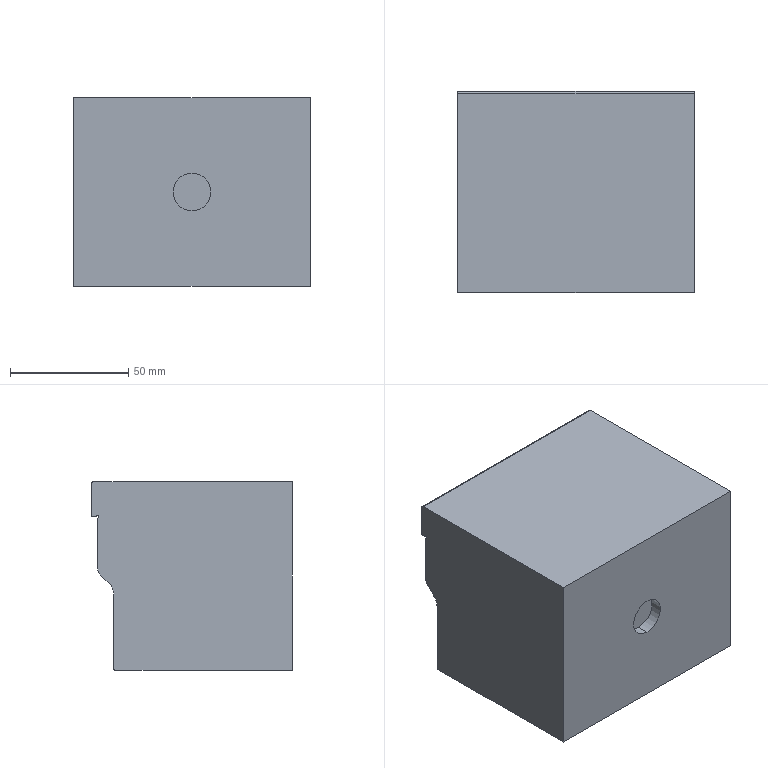Part | SolidWorks | features FlatPattern 1, ICE 1, SMBaseFlange 1, SheetMetal 1 | 1 solid | 20 faces | box 100 x 85 x 80 mm | volume 636588 mm3 | plane 11 | cylinder 9 | commonest cylinder face diameters 2 x4 16 x2 1 x1 6.4 x1 12.8 x1
STEP:
#1=CARTESIAN_POINT('',(-50.,5.,-32.));
#2=VERTEX_POINT('',#1);
#3=CARTESIAN_POINT('',(-50.,5.,-48.));
#4=VERTEX_POINT('',#3);
#5=CARTESIAN_POINT('',(-50.,5.,-40.));
#6=DIRECTION('',(0.,-1.,0.));
#7=DIRECTION('',(0.,0.,-1.));
#8=AXIS2_PLACEMENT_3D('',#5,#6,#7);
#9=CIRCLE('',#8,8.);
#10=EDGE_CURVE('',#2,#4,#9,.T.);
#11=ORIENTED_EDGE('',*,*,#10,.F.);
#12=CARTESIAN_POINT('',(-50.,0.,-32.));
#13=VERTEX_POINT('',#12);
#14=CARTESIAN_POINT('',(-50.,5.,-32.));
#15=DIRECTION('',(0.,-1.,0.));
#16=VECTOR('',#15,1000.);
#17=LINE('',#14,#16);
#18=EDGE_CURVE('',#2,#13,#17,.T.);
#19=ORIENTED_EDGE('',*,*,#18,.T.);
#20=CARTESIAN_POINT('',(-50.,0.,-48.));
#21=VERTEX_POINT('',#20);
#22=CARTESIAN_POINT('',(-50.,0.,-40.));
#23=DIRECTION('',(0.,-1.,0.));
#24=DIRECTION('',(0.,0.,-1.));
#25=AXIS2_PLACEMENT_3D('',#22,#23,#24);
#26=CIRCLE('',#25,8.);
#27=EDGE_CURVE('',#13,#21,#26,.T.);
#28=ORIENTED_EDGE('',*,*,#27,.T.);
#29=CARTESIAN_POINT('',(-50.,5.,-48.));
#30=DIRECTION('',(0.,-1.,0.));
#31=VECTOR('',#30,1000.);
#32=LINE('',#29,#31);
#33=EDGE_CURVE('',#4,#21,#32,.T.);
#34=ORIENTED_EDGE('',*,*,#33,.F.);
#35=EDGE_LOOP('',(#11,#19,#28,#34));
#36=FACE_OUTER_BOUND('',#35,.T.);
#37=CARTESIAN_POINT('',(-50.,5.,-40.));
#38=DIRECTION('',(0.,-1.,0.));
#39=DIRECTION('',(0.,0.,-1.));
#40=AXIS2_PLACEMENT_3D('',#37,#38,#39);
#41=CYLINDRICAL_SURFACE('',#40,8.);
#42=ADVANCED_FACE('',(#36),#41,.F.);
#43=CARTESIAN_POINT('',(0.,84.,0.));
#44=VERTEX_POINT('',#43);
#45=CARTESIAN_POINT('',(0.,0.,0.));
#46=VERTEX_POINT('',#45);
#47=CARTESIAN_POINT('',(0.,84.,0.));
#48=DIRECTION('',(0.,-1.,0.));
#49=VECTOR('',#48,1000.);
#50=LINE('',#47,#49);
#51=EDGE_CURVE('',#44,#46,#50,.T.);
#52=ORIENTED_EDGE('',*,*,#51,.F.);
#53=CARTESIAN_POINT('',(-100.,84.,0.));
#54=VERTEX_POINT('',#53);
#55=CARTESIAN_POINT('',(-100.,84.,0.));
#56=DIRECTION('',(1.,0.,0.));
#57=VECTOR('',#56,1000.);
#58=LINE('',#55,#57);
#59=EDGE_CURVE('',#54,#44,#58,.T.);
#60=ORIENTED_EDGE('',*,*,#59,.F.);
#61=CARTESIAN_POINT('',(-100.,0.,0.));
#62=VERTEX_POINT('',#61);
#63=CARTESIAN_POINT('',(-100.,84.,0.));
#64=DIRECTION('',(0.,-1.,0.));
#65=VECTOR('',#64,1000.);
#66=LINE('',#63,#65);
#67=EDGE_CURVE('',#54,#62,#66,.T.);
#68=ORIENTED_EDGE('',*,*,#67,.T.);
#69=CARTESIAN_POINT('',(-100.,0.,0.));
#70=DIRECTION('',(1.,0.,0.));
#71=VECTOR('',#70,1000.);
#72=LINE('',#69,#71);
#73=EDGE_CURVE('',#62,#46,#72,.T.);
#74=ORIENTED_EDGE('',*,*,#73,.T.);
#75=EDGE_LOOP('',(#52,#60,#68,#74));
#76=FACE_OUTER_BOUND('',#75,.T.);
#77=CARTESIAN_POINT('',(-100.,84.,0.));
#78=DIRECTION('',(0.,0.,1.));
#79=DIRECTION('',(0.,-1.,0.));
#80=AXIS2_PLACEMENT_3D('',#77,#78,#79);
#81=PLANE('',#80);
#82=ADVANCED_FACE('',(#76),#81,.T.);
#83=CARTESIAN_POINT('',(0.,85.,-1.));
#84=VERTEX_POINT('',#83);
#85=CARTESIAN_POINT('',(0.,84.,-1.));
#86=DIRECTION('',(1.,0.,0.));
#87=DIRECTION('',(0.,0.,-1.));
#88=AXIS2_PLACEMENT_3D('',#85,#86,#87);
#89=CIRCLE('',#88,1.);
#90=EDGE_CURVE('',#84,#44,#89,.T.);
#91=ORIENTED_EDGE('',*,*,#90,.F.);
#92=CARTESIAN_POINT('',(-100.,85.,-1.));
#93=VERTEX_POINT('',#92);
#94=CARTESIAN_POINT('',(-100.,85.,-1.));
#95=DIRECTION('',(1.,0.,0.));
#96=VECTOR('',#95,1000.);
#97=LINE('',#94,#96);
#98=EDGE_CURVE('',#93,#84,#97,.T.);
#99=ORIENTED_EDGE('',*,*,#98,.F.);
#100=CARTESIAN_POINT('',(-100.,84.,-1.));
#101=DIRECTION('',(1.,0.,0.));
#102=DIRECTION('',(0.,0.,-1.));
#103=AXIS2_PLACEMENT_3D('',#100,#101,#102);
#104=CIRCLE('',#103,1.);
#105=EDGE_CURVE('',#93,#54,#104,.T.);
#106=ORIENTED_EDGE('',*,*,#105,.T.);
#107=ORIENTED_EDGE('',*,*,#59,.T.);
#108=EDGE_LOOP('',(#91,#99,#106,#107));
#109=FACE_OUTER_BOUND('',#108,.T.);
#110=CARTESIAN_POINT('',(-100.,84.,-1.));
#111=DIRECTION('',(1.,0.,0.));
#112=DIRECTION('',(0.,0.,-1.));
#113=AXIS2_PLACEMENT_3D('',#110,#111,#112);
#114=CYLINDRICAL_SURFACE('',#113,1.);
#115=ADVANCED_FACE('',(#109),#114,.T.);
#116=CARTESIAN_POINT('',(0.,85.,-15.));
#117=VERTEX_POINT('',#116);
#118=CARTESIAN_POINT('',(0.,85.,-1.));
#119=DIRECTION('',(0.,0.,1.));
#120=VECTOR('',#119,1000.);
#121=LINE('',#118,#120);
#122=EDGE_CURVE('',#117,#84,#121,.T.);
#123=ORIENTED_EDGE('',*,*,#122,.F.);
#124=CARTESIAN_POINT('',(-100.,85.,-15.));
#125=VERTEX_POINT('',#124);
#126=CARTESIAN_POINT('',(-100.,85.,-15.));
#127=DIRECTION('',(1.,0.,0.));
#128=VECTOR('',#127,1000.);
#129=LINE('',#126,#128);
#130=EDGE_CURVE('',#125,#117,#129,.T.);
#131=ORIENTED_EDGE('',*,*,#130,.F.);
#132=CARTESIAN_POINT('',(-100.,85.,-1.));
#133=DIRECTION('',(0.,0.,1.));
#134=VECTOR('',#133,1000.);
#135=LINE('',#132,#134);
#136=EDGE_CURVE('',#125,#93,#135,.T.);
#137=ORIENTED_EDGE('',*,*,#136,.T.);
#138=ORIENTED_EDGE('',*,*,#98,.T.);
#139=EDGE_LOOP('',(#123,#131,#137,#138));
#140=FACE_OUTER_BOUND('',#139,.T.);
#141=CARTESIAN_POINT('',(-100.,85.,-1.));
#142=DIRECTION('',(0.,1.,0.));
#143=DIRECTION('',(0.,0.,1.));
#144=AXIS2_PLACEMENT_3D('',#141,#142,#143);
#145=PLANE('',#144);
#146=ADVANCED_FACE('',(#140),#145,.T.);
#147=CARTESIAN_POINT('',(0.,83.618,-15.));
#148=VERTEX_POINT('',#147);
#149=CARTESIAN_POINT('',(0.,85.,-15.));
#150=DIRECTION('',(0.,1.,0.));
#151=VECTOR('',#150,1000.);
#152=LINE('',#149,#151);
#153=EDGE_CURVE('',#148,#117,#152,.T.);
#154=ORIENTED_EDGE('',*,*,#153,.F.);
#155=CARTESIAN_POINT('',(-100.,83.618,-15.));
#156=VERTEX_POINT('',#155);
#157=CARTESIAN_POINT('',(-100.,83.618,-15.));
#158=DIRECTION('',(1.,0.,0.));
#159=VECTOR('',#158,1000.);
#160=LINE('',#157,#159);
#161=EDGE_CURVE('',#156,#148,#160,.T.);
#162=ORIENTED_EDGE('',*,*,#161,.F.);
#163=CARTESIAN_POINT('',(-100.,85.,-15.));
#164=DIRECTION('',(0.,1.,0.));
#165=VECTOR('',#164,1000.);
#166=LINE('',#163,#165);
#167=EDGE_CURVE('',#156,#125,#166,.T.);
#168=ORIENTED_EDGE('',*,*,#167,.T.);
#169=ORIENTED_EDGE('',*,*,#130,.T.);
#170=EDGE_LOOP('',(#154,#162,#168,#169));
#171=FACE_OUTER_BOUND('',#170,.T.);
#172=CARTESIAN_POINT('',(-100.,85.,-15.));
#173=DIRECTION('',(0.,0.,-1.));
#174=DIRECTION('',(0.,1.,0.));
#175=AXIS2_PLACEMENT_3D('',#172,#173,#174);
#176=PLANE('',#175);
#177=ADVANCED_FACE('',(#171),#176,.T.);
#178=CARTESIAN_POINT('',(0.,82.873,-14.667));
#179=VERTEX_POINT('',#178);
#180=CARTESIAN_POINT('',(0.,83.618,-14.));
#181=DIRECTION('',(1.,0.,0.));
#182=DIRECTION('',(0.,0.,-1.));
#183=AXIS2_PLACEMENT_3D('',#180,#181,#182);
#184=CIRCLE('',#183,1.);
#185=EDGE_CURVE('',#179,#148,#184,.T.);
#186=ORIENTED_EDGE('',*,*,#185,.F.);
#187=CARTESIAN_POINT('',(-100.,82.873,-14.667));
#188=VERTEX_POINT('',#187);
#189=CARTESIAN_POINT('',(-100.,82.873,-14.667));
#190=DIRECTION('',(1.,0.,0.));
#191=VECTOR('',#190,1000.);
#192=LINE('',#189,#191);
#193=EDGE_CURVE('',#188,#179,#192,.T.);
#194=ORIENTED_EDGE('',*,*,#193,.F.);
#195=CARTESIAN_POINT('',(-100.,83.618,-14.));
#196=DIRECTION('',(1.,0.,0.));
#197=DIRECTION('',(0.,0.,-1.));
#198=AXIS2_PLACEMENT_3D('',#195,#196,#197);
#199=CIRCLE('',#198,1.);
#200=EDGE_CURVE('',#188,#156,#199,.T.);
#201=ORIENTED_EDGE('',*,*,#200,.T.);
#202=ORIENTED_EDGE('',*,*,#161,.T.);
#203=EDGE_LOOP('',(#186,#194,#201,#202));
#204=FACE_OUTER_BOUND('',#203,.T.);
#205=CARTESIAN_POINT('',(-100.,83.618,-14.));
#206=DIRECTION('',(1.,0.,0.));
#207=DIRECTION('',(0.,0.,-1.));
#208=AXIS2_PLACEMENT_3D('',#205,#206,#207);
#209=CYLINDRICAL_SURFACE('',#208,1.);
#210=ADVANCED_FACE('',(#204),#209,.T.);
#211=CARTESIAN_POINT('',(0.,82.167,-15.373));
#212=VERTEX_POINT('',#211);
#213=CARTESIAN_POINT('',(0.,82.5,-15.));
#214=DIRECTION('',(-1.,0.,0.));
#215=DIRECTION('',(0.,0.,-1.));
#216=AXIS2_PLACEMENT_3D('',#213,#214,#215);
#217=CIRCLE('',#216,0.5);
#218=EDGE_CURVE('',#212,#179,#217,.T.);
#219=ORIENTED_EDGE('',*,*,#218,.F.);
#220=CARTESIAN_POINT('',(-100.,82.167,-15.373));
#221=VERTEX_POINT('',#220);
#222=CARTESIAN_POINT('',(-100.,82.167,-15.373));
#223=DIRECTION('',(1.,0.,0.));
#224=VECTOR('',#223,1000.);
#225=LINE('',#222,#224);
#226=EDGE_CURVE('',#221,#212,#225,.T.);
#227=ORIENTED_EDGE('',*,*,#226,.F.);
#228=CARTESIAN_POINT('',(-100.,82.5,-15.));
#229=DIRECTION('',(-1.,0.,0.));
#230=DIRECTION('',(0.,0.,-1.));
#231=AXIS2_PLACEMENT_3D('',#228,#229,#230);
#232=CIRCLE('',#231,0.5);
#233=EDGE_CURVE('',#221,#188,#232,.T.);
#234=ORIENTED_EDGE('',*,*,#233,.T.);
#235=ORIENTED_EDGE('',*,*,#193,.T.);
#236=EDGE_LOOP('',(#219,#227,#234,#235));
#237=FACE_OUTER_BOUND('',#236,.T.);
#238=CARTESIAN_POINT('',(-100.,82.5,-15.));
#239=DIRECTION('',(1.,0.,0.));
#240=DIRECTION('',(0.,0.,-1.));
#241=AXIS2_PLACEMENT_3D('',#238,#239,#240);
#242=CYLINDRICAL_SURFACE('',#241,0.5);
#243=ADVANCED_FACE('',(#237),#242,.F.);
#244=CARTESIAN_POINT('',(0.,82.5,-16.118));
#245=VERTEX_POINT('',#244);
#246=CARTESIAN_POINT('',(0.,81.5,-16.118));
#247=DIRECTION('',(1.,0.,0.));
#248=DIRECTION('',(0.,0.,1.));
#249=AXIS2_PLACEMENT_3D('',#246,#247,#248);
#250=CIRCLE('',#249,1.);
#251=EDGE_CURVE('',#245,#212,#250,.T.);
#252=ORIENTED_EDGE('',*,*,#251,.F.);
#253=CARTESIAN_POINT('',(-100.,82.5,-16.118));
#254=VERTEX_POINT('',#253);
#255=CARTESIAN_POINT('',(-100.,82.5,-16.118));
#256=DIRECTION('',(1.,0.,0.));
#257=VECTOR('',#256,1000.);
#258=LINE('',#255,#257);
#259=EDGE_CURVE('',#254,#245,#258,.T.);
#260=ORIENTED_EDGE('',*,*,#259,.F.);
#261=CARTESIAN_POINT('',(-100.,81.5,-16.118));
#262=DIRECTION('',(1.,0.,0.));
#263=DIRECTION('',(0.,0.,1.));
#264=AXIS2_PLACEMENT_3D('',#261,#262,#263);
#265=CIRCLE('',#264,1.);
#266=EDGE_CURVE('',#254,#221,#265,.T.);
#267=ORIENTED_EDGE('',*,*,#266,.T.);
#268=ORIENTED_EDGE('',*,*,#226,.T.);
#269=EDGE_LOOP('',(#252,#260,#267,#268));
#270=FACE_OUTER_BOUND('',#269,.T.);
#271=CARTESIAN_POINT('',(-100.,81.5,-16.118));
#272=DIRECTION('',(1.,0.,0.));
#273=DIRECTION('',(0.,0.,-1.));
#274=AXIS2_PLACEMENT_3D('',#271,#272,#273);
#275=CYLINDRICAL_SURFACE('',#274,1.);
#276=ADVANCED_FACE('',(#270),#275,.T.);
#277=CARTESIAN_POINT('',(0.,82.5,-36.875));
#278=VERTEX_POINT('',#277);
#279=CARTESIAN_POINT('',(0.,82.5,-16.118));
#280=DIRECTION('',(0.,0.,1.));
#281=VECTOR('',#280,1000.);
#282=LINE('',#279,#281);
#283=EDGE_CURVE('',#278,#245,#282,.T.);
#284=ORIENTED_EDGE('',*,*,#283,.F.);
#285=CARTESIAN_POINT('',(-100.,82.5,-36.875));
#286=VERTEX_POINT('',#285);
#287=CARTESIAN_POINT('',(-100.,82.5,-36.875));
#288=DIRECTION('',(1.,0.,0.));
#289=VECTOR('',#288,1000.);
#290=LINE('',#287,#289);
#291=EDGE_CURVE('',#286,#278,#290,.T.);
#292=ORIENTED_EDGE('',*,*,#291,.F.);
#293=CARTESIAN_POINT('',(-100.,82.5,-16.118));
#294=DIRECTION('',(0.,0.,1.));
#295=VECTOR('',#294,1000.);
#296=LINE('',#293,#295);
#297=EDGE_CURVE('',#286,#254,#296,.T.);
#298=ORIENTED_EDGE('',*,*,#297,.T.);
#299=ORIENTED_EDGE('',*,*,#259,.T.);
#300=EDGE_LOOP('',(#284,#292,#298,#299));
#301=FACE_OUTER_BOUND('',#300,.T.);
#302=CARTESIAN_POINT('',(-100.,82.5,-16.118));
#303=DIRECTION('',(0.,1.,0.));
#304=DIRECTION('',(0.,0.,1.));
#305=AXIS2_PLACEMENT_3D('',#302,#303,#304);
#306=PLANE('',#305);
#307=ADVANCED_FACE('',(#301),#306,.T.);
#308=CARTESIAN_POINT('',(0.,81.563,-39.137));
#309=VERTEX_POINT('',#308);
#310=CARTESIAN_POINT('',(0.,79.3,-36.875));
#311=DIRECTION('',(1.,0.,0.));
#312=DIRECTION('',(0.,0.,1.));
#313=AXIS2_PLACEMENT_3D('',#310,#311,#312);
#314=CIRCLE('',#313,3.2);
#315=EDGE_CURVE('',#309,#278,#314,.T.);
#316=ORIENTED_EDGE('',*,*,#315,.F.);
#317=CARTESIAN_POINT('',(-100.,81.563,-39.137));
#318=VERTEX_POINT('',#317);
#319=CARTESIAN_POINT('',(-100.,81.563,-39.137));
#320=DIRECTION('',(1.,0.,0.));
#321=VECTOR('',#320,1000.);
#322=LINE('',#319,#321);
#323=EDGE_CURVE('',#318,#309,#322,.T.);
#324=ORIENTED_EDGE('',*,*,#323,.F.);
#325=CARTESIAN_POINT('',(-100.,79.3,-36.875));
#326=DIRECTION('',(1.,0.,0.));
#327=DIRECTION('',(0.,0.,1.));
#328=AXIS2_PLACEMENT_3D('',#325,#326,#327);
#329=CIRCLE('',#328,3.2);
#330=EDGE_CURVE('',#318,#286,#329,.T.);
#331=ORIENTED_EDGE('',*,*,#330,.T.);
#332=ORIENTED_EDGE('',*,*,#291,.T.);
#333=EDGE_LOOP('',(#316,#324,#331,#332));
#334=FACE_OUTER_BOUND('',#333,.T.);
#335=CARTESIAN_POINT('',(-100.,79.3,-36.875));
#336=DIRECTION('',(1.,0.,0.));
#337=DIRECTION('',(0.,0.,-1.));
#338=AXIS2_PLACEMENT_3D('',#335,#336,#337);
#339=CYLINDRICAL_SURFACE('',#338,3.2);
#340=ADVANCED_FACE('',(#334),#339,.T.);
#341=CARTESIAN_POINT('',(0.,77.575,-43.125));
#342=VERTEX_POINT('',#341);
#343=CARTESIAN_POINT('',(0.,77.575,-43.125));
#344=DIRECTION('',(0.,0.7071,0.7071));
#345=VECTOR('',#344,1000.);
#346=LINE('',#343,#345);
#347=EDGE_CURVE('',#342,#309,#346,.T.);
#348=ORIENTED_EDGE('',*,*,#347,.F.);
#349=CARTESIAN_POINT('',(-100.,77.575,-43.125));
#350=VERTEX_POINT('',#349);
#351=CARTESIAN_POINT('',(-100.,77.575,-43.125));
#352=DIRECTION('',(1.,0.,0.));
#353=VECTOR('',#352,1000.);
#354=LINE('',#351,#353);
#355=EDGE_CURVE('',#350,#342,#354,.T.);
#356=ORIENTED_EDGE('',*,*,#355,.F.);
#357=CARTESIAN_POINT('',(-100.,77.575,-43.125));
#358=DIRECTION('',(0.,0.7071,0.7071));
#359=VECTOR('',#358,1000.);
#360=LINE('',#357,#359);
#361=EDGE_CURVE('',#350,#318,#360,.T.);
#362=ORIENTED_EDGE('',*,*,#361,.T.);
#363=ORIENTED_EDGE('',*,*,#323,.T.);
#364=EDGE_LOOP('',(#348,#356,#362,#363));
#365=FACE_OUTER_BOUND('',#364,.T.);
#366=CARTESIAN_POINT('',(-100.,77.575,-43.125));
#367=DIRECTION('',(0.,0.7071,-0.7071));
#368=DIRECTION('',(0.,0.7071,0.7071));
#369=AXIS2_PLACEMENT_3D('',#366,#367,#368);
#370=PLANE('',#369);
#371=ADVANCED_FACE('',(#365),#370,.T.);
#372=CARTESIAN_POINT('',(0.,75.7,-47.651));
#373=VERTEX_POINT('',#372);
#374=CARTESIAN_POINT('',(0.,82.1,-47.651));
#375=DIRECTION('',(-1.,0.,0.));
#376=DIRECTION('',(0.,0.,1.));
#377=AXIS2_PLACEMENT_3D('',#374,#375,#376);
#378=CIRCLE('',#377,6.4);
#379=EDGE_CURVE('',#373,#342,#378,.T.);
#380=ORIENTED_EDGE('',*,*,#379,.F.);
#381=CARTESIAN_POINT('',(-100.,75.7,-47.651));
#382=VERTEX_POINT('',#381);
#383=CARTESIAN_POINT('',(-100.,75.7,-47.651));
#384=DIRECTION('',(1.,0.,0.));
#385=VECTOR('',#384,1000.);
#386=LINE('',#383,#385);
#387=EDGE_CURVE('',#382,#373,#386,.T.);
#388=ORIENTED_EDGE('',*,*,#387,.F.);
#389=CARTESIAN_POINT('',(-100.,82.1,-47.651));
#390=DIRECTION('',(-1.,0.,0.));
#391=DIRECTION('',(0.,0.,1.));
#392=AXIS2_PLACEMENT_3D('',#389,#390,#391);
#393=CIRCLE('',#392,6.4);
#394=EDGE_CURVE('',#382,#350,#393,.T.);
#395=ORIENTED_EDGE('',*,*,#394,.T.);
#396=ORIENTED_EDGE('',*,*,#355,.T.);
#397=EDGE_LOOP('',(#380,#388,#395,#396));
#398=FACE_OUTER_BOUND('',#397,.T.);
#399=CARTESIAN_POINT('',(-100.,82.1,-47.651));
#400=DIRECTION('',(1.,0.,0.));
#401=DIRECTION('',(0.,0.,-1.));
#402=AXIS2_PLACEMENT_3D('',#399,#400,#401);
#403=CYLINDRICAL_SURFACE('',#402,6.4);
#404=ADVANCED_FACE('',(#398),#403,.F.);
#405=CARTESIAN_POINT('',(0.,75.7,-79.));
#406=VERTEX_POINT('',#405);
#407=CARTESIAN_POINT('',(0.,75.7,-79.));
#408=DIRECTION('',(0.,0.,1.));
#409=VECTOR('',#408,1000.);
#410=LINE('',#407,#409);
#411=EDGE_CURVE('',#406,#373,#410,.T.);
#412=ORIENTED_EDGE('',*,*,#411,.F.);
#413=CARTESIAN_POINT('',(-100.,75.7,-79.));
#414=VERTEX_POINT('',#413);
#415=CARTESIAN_POINT('',(-100.,75.7,-79.));
#416=DIRECTION('',(1.,0.,0.));
#417=VECTOR('',#416,1000.);
#418=LINE('',#415,#417);
#419=EDGE_CURVE('',#414,#406,#418,.T.);
#420=ORIENTED_EDGE('',*,*,#419,.F.);
#421=CARTESIAN_POINT('',(-100.,75.7,-79.));
#422=DIRECTION('',(0.,0.,1.));
#423=VECTOR('',#422,1000.);
#424=LINE('',#421,#423);
#425=EDGE_CURVE('',#414,#382,#424,.T.);
#426=ORIENTED_EDGE('',*,*,#425,.T.);
#427=ORIENTED_EDGE('',*,*,#387,.T.);
#428=EDGE_LOOP('',(#412,#420,#426,#427));
#429=FACE_OUTER_BOUND('',#428,.T.);
#430=CARTESIAN_POINT('',(-100.,75.7,-79.));
#431=DIRECTION('',(0.,1.,0.));
#432=DIRECTION('',(0.,0.,1.));
#433=AXIS2_PLACEMENT_3D('',#430,#431,#432);
#434=PLANE('',#433);
#435=ADVANCED_FACE('',(#429),#434,.T.);
#436=CARTESIAN_POINT('',(0.,74.7,-80.));
#437=VERTEX_POINT('',#436);
#438=CARTESIAN_POINT('',(0.,74.7,-79.));
#439=DIRECTION('',(1.,0.,0.));
#440=DIRECTION('',(0.,0.,-1.));
#441=AXIS2_PLACEMENT_3D('',#438,#439,#440);
#442=CIRCLE('',#441,1.);
#443=EDGE_CURVE('',#437,#406,#442,.T.);
#444=ORIENTED_EDGE('',*,*,#443,.F.);
#445=CARTESIAN_POINT('',(-100.,74.7,-80.));
#446=VERTEX_POINT('',#445);
#447=CARTESIAN_POINT('',(-100.,74.7,-80.));
#448=DIRECTION('',(1.,0.,0.));
#449=VECTOR('',#448,1000.);
#450=LINE('',#447,#449);
#451=EDGE_CURVE('',#446,#437,#450,.T.);
#452=ORIENTED_EDGE('',*,*,#451,.F.);
#453=CARTESIAN_POINT('',(-100.,74.7,-79.));
#454=DIRECTION('',(1.,0.,0.));
#455=DIRECTION('',(0.,0.,-1.));
#456=AXIS2_PLACEMENT_3D('',#453,#454,#455);
#457=CIRCLE('',#456,1.);
#458=EDGE_CURVE('',#446,#414,#457,.T.);
#459=ORIENTED_EDGE('',*,*,#458,.T.);
#460=ORIENTED_EDGE('',*,*,#419,.T.);
#461=EDGE_LOOP('',(#444,#452,#459,#460));
#462=FACE_OUTER_BOUND('',#461,.T.);
#463=CARTESIAN_POINT('',(-100.,74.7,-79.));
#464=DIRECTION('',(1.,0.,0.));
#465=DIRECTION('',(0.,0.,-1.));
#466=AXIS2_PLACEMENT_3D('',#463,#464,#465);
#467=CYLINDRICAL_SURFACE('',#466,1.);
#468=ADVANCED_FACE('',(#462),#467,.T.);
#469=CARTESIAN_POINT('',(0.,0.,-80.));
#470=VERTEX_POINT('',#469);
#471=CARTESIAN_POINT('',(0.,0.,-80.));
#472=DIRECTION('',(0.,1.,0.));
#473=VECTOR('',#472,1000.);
#474=LINE('',#471,#473);
#475=EDGE_CURVE('',#470,#437,#474,.T.);
#476=ORIENTED_EDGE('',*,*,#475,.F.);
#477=CARTESIAN_POINT('',(-100.,0.,-80.));
#478=VERTEX_POINT('',#477);
#479=CARTESIAN_POINT('',(-100.,0.,-80.));
#480=DIRECTION('',(1.,0.,0.));
#481=VECTOR('',#480,1000.);
#482=LINE('',#479,#481);
#483=EDGE_CURVE('',#478,#470,#482,.T.);
#484=ORIENTED_EDGE('',*,*,#483,.F.);
#485=CARTESIAN_POINT('',(-100.,0.,-80.));
#486=DIRECTION('',(0.,1.,0.));
#487=VECTOR('',#486,1000.);
#488=LINE('',#485,#487);
#489=EDGE_CURVE('',#478,#446,#488,.T.);
#490=ORIENTED_EDGE('',*,*,#489,.T.);
#491=ORIENTED_EDGE('',*,*,#451,.T.);
#492=EDGE_LOOP('',(#476,#484,#490,#491));
#493=FACE_OUTER_BOUND('',#492,.T.);
#494=CARTESIAN_POINT('',(-100.,0.,-80.));
#495=DIRECTION('',(0.,0.,-1.));
#496=DIRECTION('',(-1.,0.,0.));
#497=AXIS2_PLACEMENT_3D('',#494,#495,#496);
#498=PLANE('',#497);
#499=ADVANCED_FACE('',(#493),#498,.T.);
#500=CARTESIAN_POINT('',(-50.,0.,-40.));
#501=DIRECTION('',(0.,-1.,0.));
#502=DIRECTION('',(0.,0.,-1.));
#503=AXIS2_PLACEMENT_3D('',#500,#501,#502);
#504=CIRCLE('',#503,8.);
#505=EDGE_CURVE('',#21,#13,#504,.T.);
#506=ORIENTED_EDGE('',*,*,#505,.F.);
#507=ORIENTED_EDGE('',*,*,#27,.F.);
#508=EDGE_LOOP('',(#506,#507));
#509=FACE_BOUND('',#508,.T.);
#510=CARTESIAN_POINT('',(0.,0.,0.));
#511=DIRECTION('',(0.,0.,-1.));
#512=VECTOR('',#511,1000.);
#513=LINE('',#510,#512);
#514=EDGE_CURVE('',#46,#470,#513,.T.);
#515=ORIENTED_EDGE('',*,*,#514,.F.);
#516=ORIENTED_EDGE('',*,*,#73,.F.);
#517=CARTESIAN_POINT('',(-100.,0.,0.));
#518=DIRECTION('',(0.,0.,-1.));
#519=VECTOR('',#518,1000.);
#520=LINE('',#517,#519);
#521=EDGE_CURVE('',#62,#478,#520,.T.);
#522=ORIENTED_EDGE('',*,*,#521,.T.);
#523=ORIENTED_EDGE('',*,*,#483,.T.);
#524=EDGE_LOOP('',(#515,#516,#522,#523));
#525=FACE_OUTER_BOUND('',#524,.T.);
#526=CARTESIAN_POINT('',(-100.,0.,0.));
#527=DIRECTION('',(0.,-1.,0.));
#528=DIRECTION('',(0.,0.,-1.));
#529=AXIS2_PLACEMENT_3D('',#526,#527,#528);
#530=PLANE('',#529);
#531=ADVANCED_FACE('',(#509,#525),#530,.T.);
#532=ORIENTED_EDGE('',*,*,#67,.F.);
#533=ORIENTED_EDGE('',*,*,#105,.F.);
#534=ORIENTED_EDGE('',*,*,#136,.F.);
#535=ORIENTED_EDGE('',*,*,#167,.F.);
#536=ORIENTED_EDGE('',*,*,#200,.F.);
#537=ORIENTED_EDGE('',*,*,#233,.F.);
#538=ORIENTED_EDGE('',*,*,#266,.F.);
#539=ORIENTED_EDGE('',*,*,#297,.F.);
#540=ORIENTED_EDGE('',*,*,#330,.F.);
#541=ORIENTED_EDGE('',*,*,#361,.F.);
#542=ORIENTED_EDGE('',*,*,#394,.F.);
#543=ORIENTED_EDGE('',*,*,#425,.F.);
#544=ORIENTED_EDGE('',*,*,#458,.F.);
#545=ORIENTED_EDGE('',*,*,#489,.F.);
#546=ORIENTED_EDGE('',*,*,#521,.F.);
#547=EDGE_LOOP('',(#532,#533,#534,#535,#536,#537,#538,#539,#540,#541,#542,#543,#544,#545,#546));
#548=FACE_OUTER_BOUND('',#547,.T.);
#549=CARTESIAN_POINT('',(-100.,74.7,-79.));
#550=DIRECTION('',(1.,0.,0.));
#551=DIRECTION('',(0.,0.,-1.));
#552=AXIS2_PLACEMENT_3D('',#549,#550,#551);
#553=PLANE('',#552);
#554=ADVANCED_FACE('',(#548),#553,.F.);
#555=ORIENTED_EDGE('',*,*,#51,.T.);
#556=ORIENTED_EDGE('',*,*,#514,.T.);
#557=ORIENTED_EDGE('',*,*,#475,.T.);
#558=ORIENTED_EDGE('',*,*,#443,.T.);
#559=ORIENTED_EDGE('',*,*,#411,.T.);
#560=ORIENTED_EDGE('',*,*,#379,.T.);
#561=ORIENTED_EDGE('',*,*,#347,.T.);
#562=ORIENTED_EDGE('',*,*,#315,.T.);
#563=ORIENTED_EDGE('',*,*,#283,.T.);
#564=ORIENTED_EDGE('',*,*,#251,.T.);
#565=ORIENTED_EDGE('',*,*,#218,.T.);
#566=ORIENTED_EDGE('',*,*,#185,.T.);
#567=ORIENTED_EDGE('',*,*,#153,.T.);
#568=ORIENTED_EDGE('',*,*,#122,.T.);
#569=ORIENTED_EDGE('',*,*,#90,.T.);
#570=EDGE_LOOP('',(#555,#556,#557,#558,#559,#560,#561,#562,#563,#564,#565,#566,#567,#568,#569));
#571=FACE_OUTER_BOUND('',#570,.T.);
#572=CARTESIAN_POINT('',(0.,74.7,-79.));
#573=DIRECTION('',(1.,0.,0.));
#574=DIRECTION('',(0.,0.,-1.));
#575=AXIS2_PLACEMENT_3D('',#572,#573,#574);
#576=PLANE('',#575);
#577=ADVANCED_FACE('',(#571),#576,.T.);
#578=ORIENTED_EDGE('',*,*,#18,.F.);
#579=CARTESIAN_POINT('',(-50.,5.,-40.));
#580=DIRECTION('',(0.,-1.,0.));
#581=DIRECTION('',(0.,0.,-1.));
#582=AXIS2_PLACEMENT_3D('',#579,#580,#581);
#583=CIRCLE('',#582,8.);
#584=EDGE_CURVE('',#4,#2,#583,.T.);
#585=ORIENTED_EDGE('',*,*,#584,.F.);
#586=ORIENTED_EDGE('',*,*,#33,.T.);
#587=ORIENTED_EDGE('',*,*,#505,.T.);
#588=EDGE_LOOP('',(#578,#585,#586,#587));
#589=FACE_OUTER_BOUND('',#588,.T.);
#590=CARTESIAN_POINT('',(-50.,5.,-40.));
#591=DIRECTION('',(0.,-1.,0.));
#592=DIRECTION('',(0.,0.,-1.));
#593=AXIS2_PLACEMENT_3D('',#590,#591,#592);
#594=CYLINDRICAL_SURFACE('',#593,8.);
#595=ADVANCED_FACE('',(#589),#594,.F.);
#596=ORIENTED_EDGE('',*,*,#584,.T.);
#597=ORIENTED_EDGE('',*,*,#10,.T.);
#598=EDGE_LOOP('',(#596,#597));
#599=FACE_OUTER_BOUND('',#598,.T.);
#600=CARTESIAN_POINT('',(-50.,5.,-40.));
#601=DIRECTION('',(0.,-1.,0.));
#602=DIRECTION('',(0.,0.,-1.));
#603=AXIS2_PLACEMENT_3D('',#600,#601,#602);
#604=PLANE('',#603);
#605=ADVANCED_FACE('',(#599),#604,.T.);
#606=CLOSED_SHELL('',(#42,#82,#115,#146,#177,#210,#243,#276,#307,#340,#371,#404,#435,#468,#499,#531,#554,#577,#595,#605));
#607=MANIFOLD_SOLID_BREP('',#606);
#608=CARTESIAN_POINT('',(0.,0.,0.));
#609=DIRECTION('',(0.,0.,1.));
#610=DIRECTION('',(1.,0.,0.));
#611=AXIS2_PLACEMENT_3D('',#608,#609,#610);
#612=(LENGTH_UNIT()NAMED_UNIT(*)SI_UNIT(.MILLI.,.METRE.));
#613=UNCERTAINTY_MEASURE_WITH_UNIT(LENGTH_MEASURE(0.00001),#612,'','');
#614=(NAMED_UNIT(*)PLANE_ANGLE_UNIT()SI_UNIT($,.RADIAN.));
#615=(NAMED_UNIT(*)SI_UNIT($,.STERADIAN.)SOLID_ANGLE_UNIT());
#616=(GEOMETRIC_REPRESENTATION_CONTEXT(3)GLOBAL_UNCERTAINTY_ASSIGNED_CONTEXT((#613))GLOBAL_UNIT_ASSIGNED_CONTEXT((#612,#614,#615))REPRESENTATION_CONTEXT('',''));
#617=ADVANCED_BREP_SHAPE_REPRESENTATION('',(#607,#611),#616);